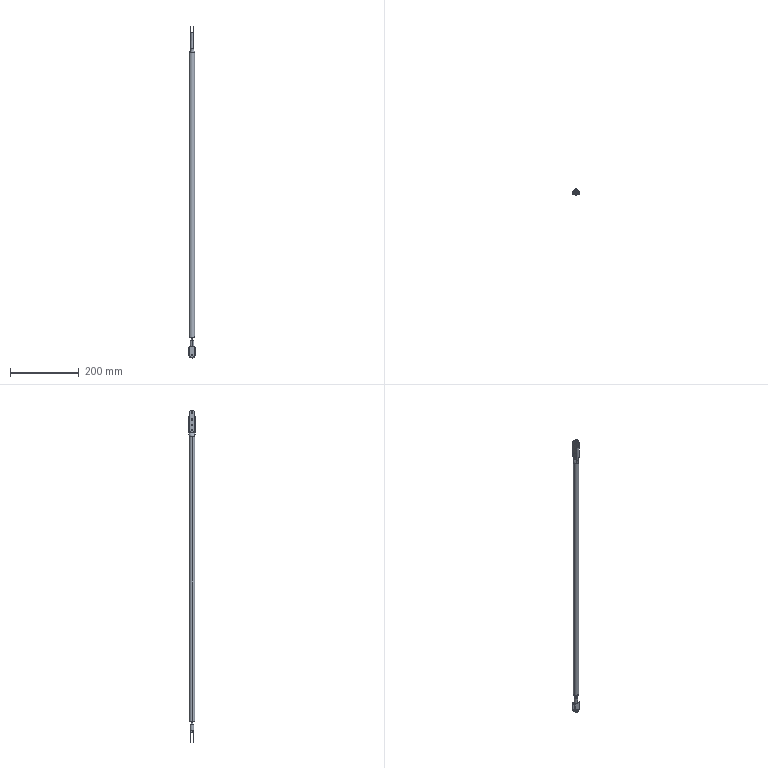Part | SolidWorks | features BaseBody 3 | 3 solids | 96 faces | box 18 x 19.559 x 964 mm | volume 45186 mm3 | cylinder 49 | plane 28 | spline 14 | cone 5 | commonest cylinder face diameters 3.175 x12 4 x8 15 x6 4.826 x4 4.9 x4 6.858 x3